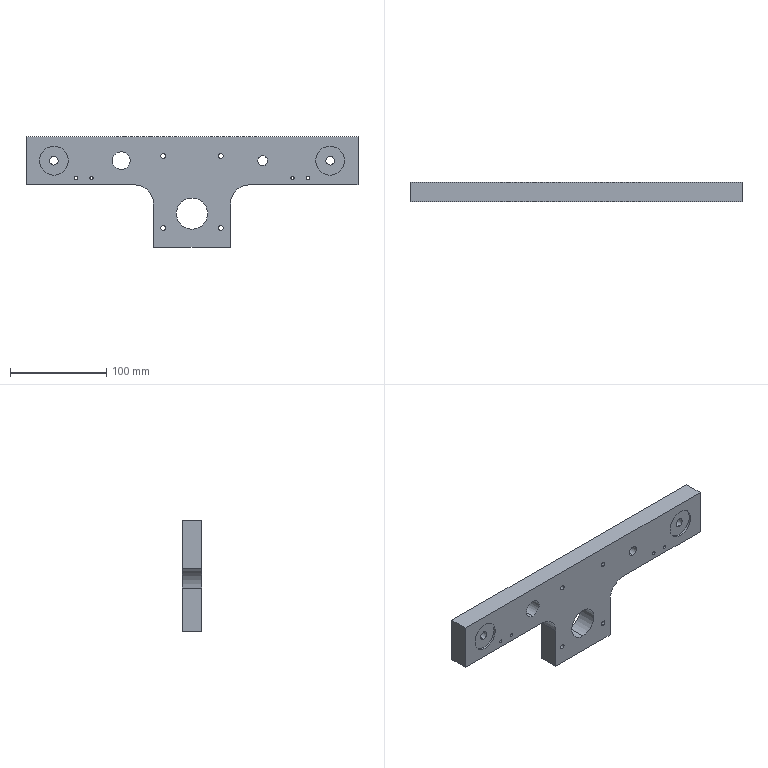Part | STEP file | 11-FG-SJ00711 | 1 solid | 50 faces | box 345 x 20 x 115 mm | volume 419514 mm3 | cylinder 36 | plane 14 | commonest cylinder face diameters 3.3 x8 5 x8 9 x4 15 x4 30 x4 10.2 x2